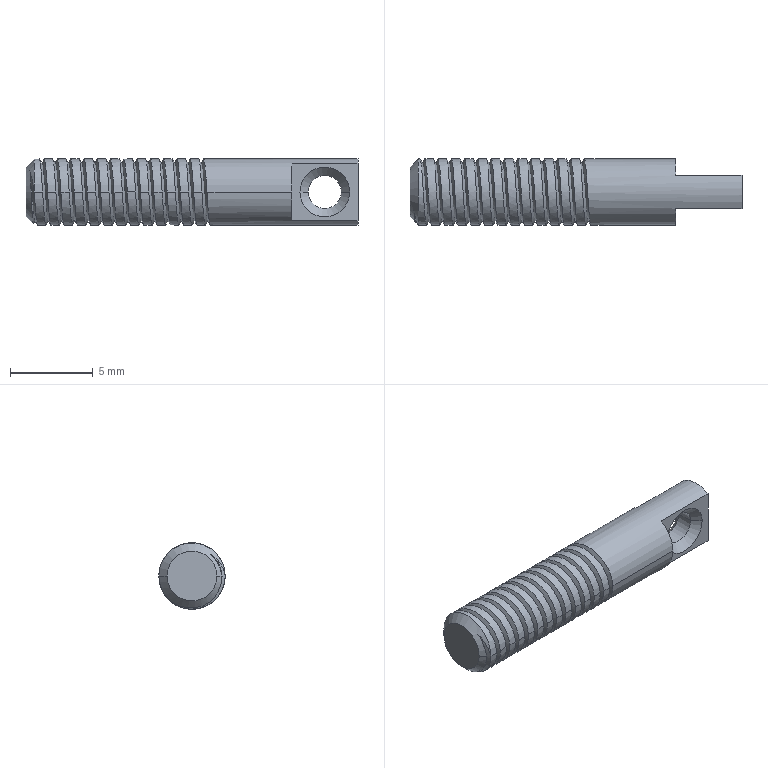Part | NX | 1 solid | 52 faces | box 20 x 4 x 4 mm | volume 215.781 mm3 | cylinder 31 | spline 8 | plane 7 | cone 6 | commonest cylinder face diameters 4 x29 2 x2